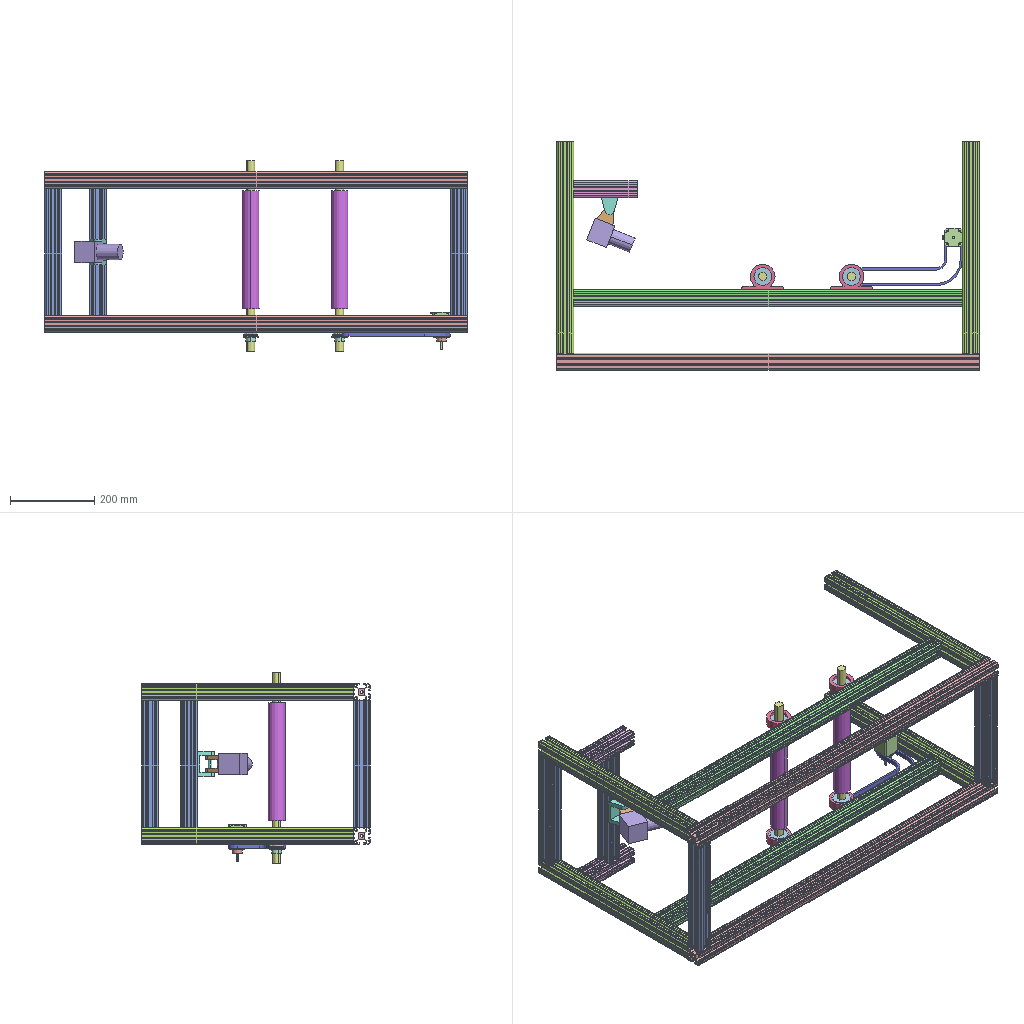Assembly | SolidWorks | 17 different items | 35 placed | box 1000 x 540 x 450 mm
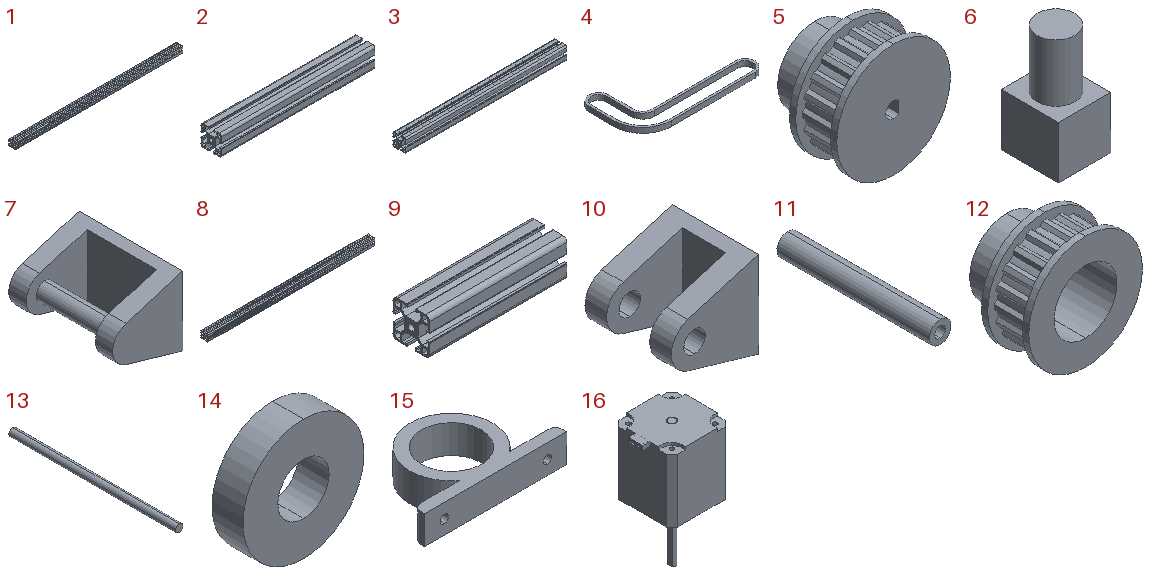Parts list (item | name | quantity | size | volume | features):
1 | - | x2 | 1000 x 40 x 40 mm | 576545 mm3 | features WeldMemberFeat 1, WeldmentFeature 1
2 | - | x4 | 300 x 40 x 40 mm | 172964 mm3 | features WeldMemberFeat 1, WeldmentFeature 1
3 | - | x4 | 500 x 40 x 40 mm | 288273 mm3 | features WeldMemberFeat 1, WeldmentFeature 1
4 | - | x1 | 260.844 x 135.477 x 11 mm | 38829 mm3 | features Extrusion 1
5 | - | x1 | 36 x 25 x 36 mm | 16244 mm3 | features ICE 5, Extrusion 1, Fillet 1
6 | - | x1 | 50 x 55 x 105 mm | 194665 mm3 | features Extrusion 1, ICE 1
7 | - | x1 | 40.645 x 60 x 40 mm | 33727 mm3 | features ICE 2, Extrusion 1
8 | - | x2 | 920 x 40 x 40 mm | 530422 mm3 | features WeldMemberFeat 1, WeldmentFeature 1
9 | - | x2 | 150 x 40 x 40 mm | 86482 mm3 | features WeldMemberFeat 1, WeldmentFeature 1
10 | - | x1 | 40.645 x 40 x 40 mm | 24880 mm3 | features ICE 2, Extrusion 1
11 | - | x2 | 40 x 280 x 40 mm | 263894 mm3 | features Extrusion 1
12 | - | x2 | 36 x 25 x 36 mm | 8830 mm3 | features ICE 5, Extrusion 1, Fillet 1
13 | - | x2 | 20 x 450 x 20 mm | 141372 mm3 | features Extrusion 1
14 | - | x4 | 47 x 12 x 47 mm | 17049 mm3 | features Extrusion 1
15 | - | x4 | 100 x 60.381 x 20 mm | 38212 mm3 | features ICE 3, Extrusion 1, Fillet 1
16 | - | x1 | 47 x 42 x 89 mm | 81069 mm3 | features ICE 8, Extrusion 1
17 | Bearing Bracket | x1 | - | - | -
Mates (type | each side: item.copy, entity, surface, feature):
Coincident | 1.1 face plane Aluminum profile 40 X 40B X R4.5(1) | 2.1 face plane Aluminum profile 40 X 40B X R4.5(1) | 3 times
Coincident | 2.1 face plane Aluminum profile 40 X 40B X R4.5(1) | 1.2 face plane Aluminum profile 40 X 40B X R4.5(1) | 3 times
Coincident | 1.1 face plane Aluminum profile 40 X 40B X R4.5(1) | 3.1 face plane Aluminum profile 40 X 40B X R4.5(1) | 3 times
Coincident | 1.2 face plane Aluminum profile 40 X 40B X R4.5(1) | 3.2 face plane Aluminum profile 40 X 40B X R4.5(1) | 3 times
Coincident | 3.1 face plane Aluminum profile 40 X 40B X R4.5(1) | 2.2 face plane Aluminum profile 40 X 40B X R4.5(1) | 2 times
Coincident | 3.2 face plane Aluminum profile 40 X 40B X R4.5(1) | 2.2 face plane Aluminum profile 40 X 40B X R4.5(1)
Coincident | 3.1 face plane Aluminum profile 40 X 40B X R4.5(1) | 9.1 face plane Aluminum profile 40 X 40B X R4.5(1) | 2 times
Coincident | 3.2 face plane Aluminum profile 40 X 40B X R4.5(1) | 9.2 face plane Aluminum profile 40 X 40B X R4.5(1) | 2 times
Coincident | 9.1 face plane Aluminum profile 40 X 40B X R4.5(1) | 9.2 face plane Aluminum profile 40 X 40B X R4.5(1)
Coincident | 9.2 face plane Aluminum profile 40 X 40B X R4.5(1) | 2.3 face plane Aluminum profile 40 X 40B X R4.5(1)
Coincident | 9.1 face plane Aluminum profile 40 X 40B X R4.5(1) | 2.3 face plane Aluminum profile 40 X 40B X R4.5(1)
DistanceDim | 2.3 face plane Aluminum profile 40 X 40B X R4.5(1) | 9.2 face plane Aluminum profile 40 X 40B X R4.5(1)
Coincident | 2.3 face plane Aluminum profile 40 X 40B X R4.5(1) | 7.1 face plane Boss-Extrude1
Coincident | 2.3 face plane Aluminum profile 40 X 40B X R4.5(1) | 7.1 edge
DistanceDim | 7.1 face plane Boss-Extrude1 | 9.2 face plane Aluminum profile 40 X 40B X R4.5(1)
Coincident | 7.1 face plane Cut-Extrude1 | 10.1 face plane Boss-Extrude1
Coincident | 7.1 face cylinder Boss-Extrude2 | 10.1 edge
Coincident | 1.1 face plane Aluminum profile 40 X 40B X R4.5(1) | 3.3 face plane Aluminum profile 40 X 40B X R4.5(1) | 2 times
Coincident | 1.2 face plane Aluminum profile 40 X 40B X R4.5(1) | 3.4 face plane Aluminum profile 40 X 40B X R4.5(1) | 3 times
Coincident | 1.2 face plane Aluminum profile 40 X 40B X R4.5(1) | 2.4 face plane Aluminum profile 40 X 40B X R4.5(1) | 2 times
Coincident | 1.1 face plane Aluminum profile 40 X 40B X R4.5(1) | 2.4 face plane Aluminum profile 40 X 40B X R4.5(1)
Coincident | 10.1 face plane Boss-Extrude1 | 6.1 face plane Boss-Extrude1
DistanceDim | 10.1 edge | 6.1 edge | 2 times
Coincident | 3.2 face plane Aluminum profile 40 X 40B X R4.5(1) | 8.1 face plane Aluminum profile 40 X 40B X R4.5(1) | 2 times
Coincident | 8.2 face plane Aluminum profile 40 X 40B X R4.5(1) | 8.1 face plane Aluminum profile 40 X 40B X R4.5(1)
Coincident | 8.2 edge | 15.1 face plane Boss-Extrude1
DistanceDim | 15.1 face plane Boss-Extrude1 | 8.2 face plane Aluminum profile 40 X 40B X R4.5(1)
Coincident | 8.1 face plane Aluminum profile 40 X 40B X R4.5(1) | 15.2 face plane Boss-Extrude1
DistanceDim | 15.2 face plane Boss-Extrude1 | 8.1 face plane Aluminum profile 40 X 40B X R4.5(1)
Coincident | 15.1 edge | 15.2 edge
Coincident | 15.1 face plane Boss-Extrude1 | 14.1 face plane Boss-Extrude1
Concentric | 15.1 face cylinder Cut-Extrude2 | 14.1 face cylinder Boss-Extrude1
Coincident | 15.2 face plane Boss-Extrude1 | 14.2 face plane Boss-Extrude1
Concentric | 15.2 face cylinder Cut-Extrude2 | 14.2 face cylinder Boss-Extrude1
Concentric | 14.1 face cylinder Boss-Extrude1 | 13.1 face cylinder Boss-Extrude1
Concentric | 13.1 face cylinder Boss-Extrude1 | 11.1 face cylinder Boss-Extrude1
Concentric | 13.1 face cylinder Boss-Extrude1 | 12.1 face cylinder Cut-Extrude3
Coincident | 8.2 face plane Aluminum profile 40 X 40B X R4.5(1) | 15.3 face plane Boss-Extrude1
Coincident | 15.1 face plane Boss-Extrude1 | 15.3 face plane Boss-Extrude1
Coincident | 8.1 face plane Aluminum profile 40 X 40B X R4.5(1) | 15.4 face plane Boss-Extrude1
Coincident | 15.2 face plane Boss-Extrude1 | 15.4 face plane Boss-Extrude1
Coincident | 15.3 edge | 15.4 edge
Coincident | 15.4 face plane Boss-Extrude1 | 14.3 face plane Boss-Extrude1
Concentric | 15.4 face cylinder Cut-Extrude2 | 14.3 face cylinder Boss-Extrude1
Coincident | 15.3 face plane Boss-Extrude1 | 14.4 face plane Boss-Extrude1
Concentric | 15.3 face cylinder Cut-Extrude2 | 14.4 face cylinder Boss-Extrude1
Concentric | 14.4 face cylinder Boss-Extrude1 | 13.2 face cylinder Boss-Extrude1
Coincident | 13.1 face plane Boss-Extrude1 | 13.2 face plane Boss-Extrude1
Concentric | 13.2 face cylinder Boss-Extrude1 | 11.2 face cylinder Boss-Extrude1
Coincident | 11.1 face plane Boss-Extrude1 | 11.2 face plane Boss-Extrude1
Concentric | 13.2 face cylinder Boss-Extrude1 | 12.2 face cylinder Cut-Extrude3
Coincident | 12.1 face plane Boss-Extrude4 | 12.2 face plane Boss-Extrude4
Coincident | 12.1 face plane Boss-Extrude2 | 5.1 face plane Boss-Extrude2
Concentric | 5.1 face cylinder Boss-Extrude1 | 4.1 face cylinder Boss-Extrude1
Coincident | 5.1 face plane Boss-Extrude2 | 4.1 face plane Boss-Extrude1
Coincident | 3.3 face plane Aluminum profile 40 X 40B X R4.5(1) | 3.4 face plane Aluminum profile 40 X 40B X R4.5(1)
Coincident | 3.3 face plane Aluminum profile 40 X 40B X R4.5(1) | 16.1 face plane Boss-Extrude1 | 2 times
Concentric | 5.1 face cylinder Cut-Extrude3 | 16.1 face cylinder Boss-Extrude3
Parallel | 8.2 face plane Aluminum profile 40 X 40B X R4.5(1) | 4.1 face plane Boss-Extrude1
Coincident | 3.1 face plane Aluminum profile 40 X 40B X R4.5(1) | 8.2 face plane Aluminum profile 40 X 40B X R4.5(1) | 2 times
Tangent | 12.1 face cylinder Boss-Extrude1 | 4.1 face plane Boss-Extrude1